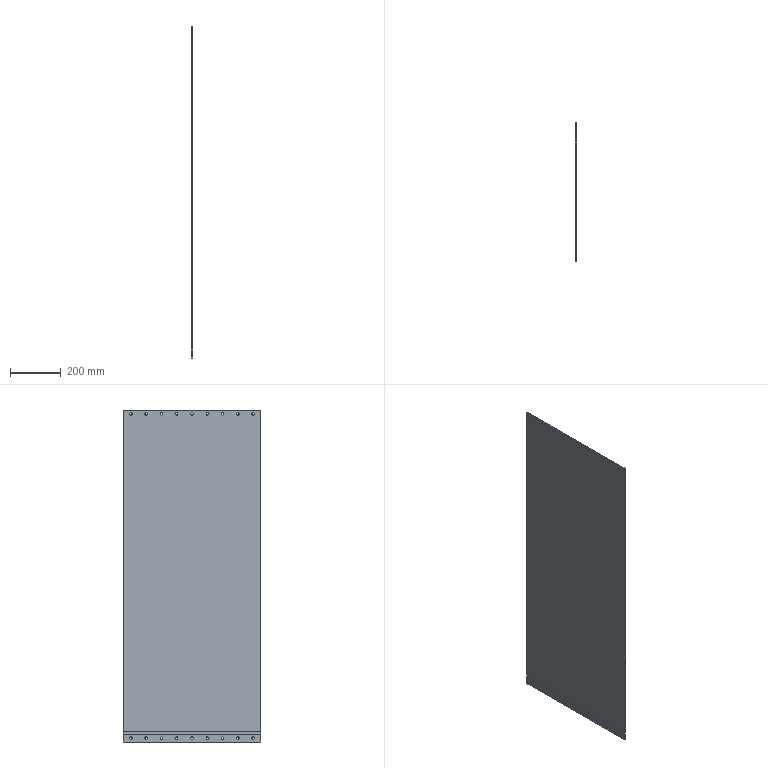Part | SolidWorks | features HoleWzd 2, LPattern 2, EdgeFlange 1, FlatPattern 1, SMBaseFlange 1, SheetMetal 1, UnFold 1, WeldmentFeature 1 | 1 solid | 50 faces | box 4 x 540 x 1303 mm | volume 2808816 mm3 | cylinder 36 | plane 14 | commonest cylinder face diameters 10 x36